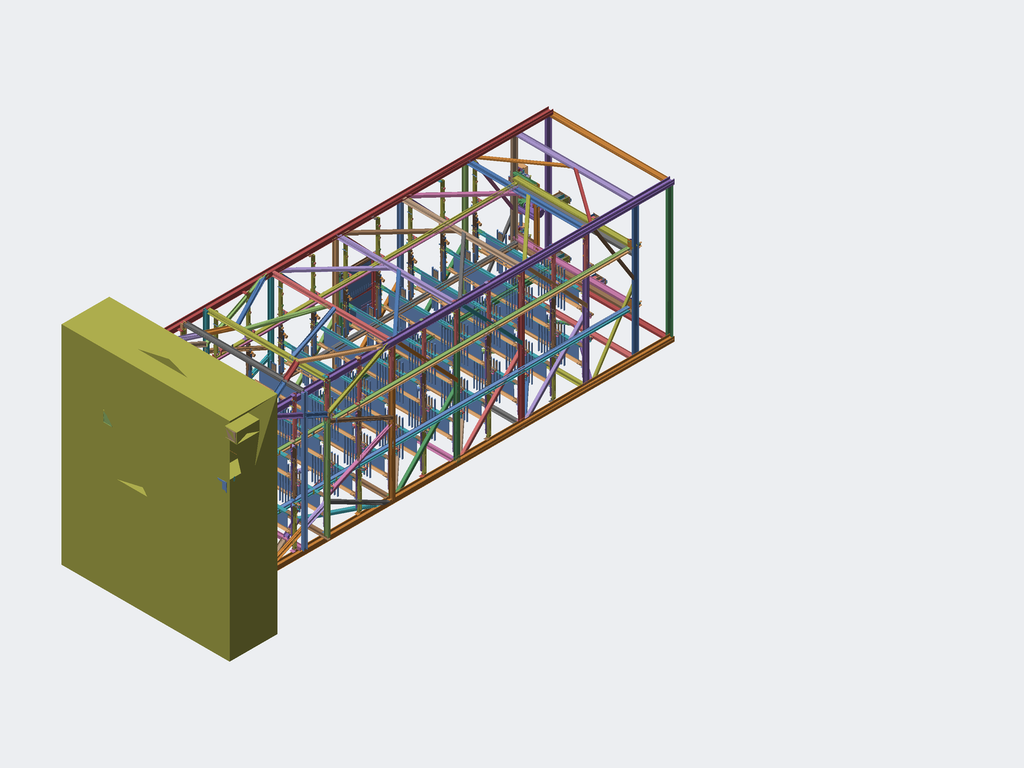Assembly | STEP file | 288 different items | 17335 placed
Parts list (item | name | quantity | parent item | size | volume):
1 | 01-Cross beam H150X150_default<machining> | x1 | in Main drive platform | 3170 x 150 x 150 mm | 12529220 mm3
2 | 01-Cross beam H150X150_default<machining> | x1 | in Main drive platform | 3170 x 150 x 150 mm | 12568854 mm3
3 | 02-Longitudinal beam H150X150_default<machining> | x1 | in Main drive platform | 1243 x 150 x 150 mm | 4402012 mm3
4 | 02-Longitudinal beam H150X150_default<machining> | x1 | in Main drive platform | 1243 x 150 x 150 mm | 4402012 mm3
5 | 02-Longitudinal beam H150X150_default<machining> | x1 | in Main drive platform | 1243 x 150 x 150 mm | 4482817 mm3
6 | 02-Longitudinal beam H150X150_default<machining> | x1 | in Main drive platform | 1243 x 150 x 150 mm | 4398211 mm3
7 | 02-Longitudinal beam H150X150_default<machining> | x1 | in Main drive platform | 1243 x 150 x 150 mm | 4398211 mm3
8 | Motor fixing plate | x1 | in Main drive platform | 370 x 435 x 20 mm | 3150576 mm3
9 | Bearing seat fixing plate | x2 | in Main drive platform | 470 x 360 x 20 mm | 3025589 mm3
10 | Counterweight hanging seat | x2 | in Main drive platform | 250 x 120 x 120 mm | 1060691 mm3
11 | 05 Rib plate | x4 | in Main drive platform | 176 x 140 x 10 mm | 160140 mm3
12 | 07 Rib plate | x2 | in Main drive platform | 156 x 140 x 10 mm | 146140 mm3
13 | 08 Rib plate | x2 | in Main drive platform | 166 x 140 x 10 mm | 153140 mm3
14 | 06 Rib plate | x4 | in Main drive platform | 71 x 128 x 10 mm | 86880 mm3
15 | 05-Base plate | x2 | in Sprocket seat | 360 x 470 x 16 mm | 2420472 mm3
16 | 04-Vertical plate | x4 | in Sprocket seat | 460 x 159 x 10 mm | 651900 mm3
17 | 03-Rib plate | x8 | in Sprocket seat | 152 x 159 x 10 mm | 208755 mm3
18 | 02-Top plate | x2 | in Sprocket seat | 460 x 550 x 16 mm | 3248676 mm3
19 | 01-Pad plate | x2 | in Sprocket seat | 148 x 110 x 6 mm | 92855 mm3
20 | 01-Pad plate | x2 | in Sprocket seat | 148 x 110 x 6 mm | 92855 mm3
21 | 01-Pad plate | x2 | in Sprocket seat | 148 x 110 x 6 mm | 92855 mm3
22 | 01-Pad plate | x2 | in Sprocket seat | 148 x 110 x 6 mm | 92855 mm3
23 | 06-Base plate | x8 | in Sprocket seat | 130 x 70 x 16 mm | 143137 mm3
24 | GB/T7810-1995 pillow block bearing UCP318 | x4 | in Drive mechanism assembly | 430 x 242.58 x 111.692 mm | 3436348 mm3
25 | 01-Main drive shaft | x2 | in Drive mechanism assembly | 1190 x 100 x 100 mm | 8433276 mm3
26 | Internal ring gear m=4  Z=56 | x2 | in CL7 Assembly | 180.99 x 350 x 350 mm | 2653491 mm3
27 | Internal ring gear A m=4  Z=56 | x2 | in CL7 Assembly | 177 x 350 x 350 mm | 2601765 mm3
28 | External ring gear m=4  Z=56 | x4 | in CL7 Assembly | 160.5 x 231.789 x 231.789 mm | 3084589 mm3
29 | Retaining ring | x4 | in CL7 Assembly | 19 x 240 x 240 mm | 192307 mm3
30 | Seal ring | x4 | in CL7 Assembly | 15.499 x 219.997 x 219.997 mm | 158146 mm3
31 | - | x4 | in CL7 Assembly | 3 x 239 x 239 mm | 65691 mm3
32 | Expansion ring | x4 | in CL7 Assembly | 245.982 x 245.031 x 3.5 mm | 25663 mm3
33 | Bolt M20x85 | x20 | in CL7 Assembly | 96 x 31.2 x 27.02 mm | 34962 mm3
34 | Grease fitting_M10X1_45 | x2 | in CL7 Assembly | 12 x 16.561 x 25.211 mm | 1753 mm3
35 | 03-Main drive sprocket | x2 | in Drive mechanism assembly | 232.271 x 231.883 x 162 mm | 2819895 mm3
36 | 02-Spacer | x4 | in Drive mechanism assembly | 100 x 100 x 22 mm | 32545 mm3
37 | Anti-jump chain bracket | x2 | in Drive mechanism assembly | 448 x 66 x 174 mm | 570819 mm3
38 | Chain press plate | x8 | in Drive mechanism assembly | 174 x 174 x 20 mm | 359243 mm3
39 | Anti-jump chain fixing seat | x1 | in Drive mechanism assembly | 550 x 308 x 360 mm | 1812248 mm3
40 | - | x2 | in Drive mechanism assembly | 70 x 27.713 x 24 mm | 16944 mm3
41 | - | x2 | in Drive mechanism assembly | 26.17 x 22.664 x 15.9 mm | 3864 mm3
42 | 01-Base plate | x2 | in Driven sprocket seat 1 | 420 x 16 x 435 mm | 2578914 mm3
43 | 03-Vertical plate | x2 | in Driven sprocket seat 1 | 420 x 204 x 16 mm | 1184293 mm3
44 | 03-Vertical plate | x2 | in Driven sprocket seat 1 | 420 x 204 x 16 mm | 1184293 mm3
45 | 02-Rib plate | x8 | in Driven sprocket seat 1 | 89 x 204 x 8 mm | 93564 mm3
46 | 04-Rib plate | x2 | in Driven sprocket seat 1 | 80 x 225 x 8 mm | 142200 mm3
47 | 04-Driven shaft 1 | x2 | in Driven sprocket assembly 1 | 305 x 60 x 60 mm | 857375 mm3
48 | PCSL50T-5300-03-Driven sprocket 1 | x2 | in Driven sprocket assembly 1 | 232.271 x 231.883 x 165 mm | 2210784 mm3
49 | GB/T276-94 deep groove ball bearing 6212-2Z | x8 | in Driven sprocket assembly 1, Driven sprocket assembly 2 | 22 x 110 x 110 mm | 94070 mm3
50 | GB893.1-86 hole elastic retaining ring type A 110 | x8 | in Driven sprocket assembly 1, Driven sprocket assembly 2 | 117 x 115.007 x 3 mm | 6744 mm3
51 | 05-Spacer 1 | x4 | in Driven sprocket assembly 1 | 70 x 70 x 39 mm | 39820 mm3
52 | Driven chain press plate 1 | x4 | in Driven sprocket assembly 1 | 130 x 170 x 20 mm | 254830 mm3
53 | Driven chain anti-jump bracket 1 | x2 | in Driven sprocket assembly 1 | 225 x 66 x 220 mm | 431717 mm3
54 | JBZQ4348-1997 shaft end baffle 60 | x8 | in Driven sprocket assembly 1, Driven sprocket assembly 2 | 130 x 40 x 8 mm | 37528 mm3
55 | Anti-jump chain fixing seat 1 | x1 | in Drive mechanism assembly | 550 x 308 x 360 mm | 1812248 mm3
56 | Counterweight connecting plate_default<machining> | x2 | in Drive mechanism assembly | 196 x 135 x 65 mm | 585213 mm3
57 | Chain joint | x8 | in Drive mechanism assembly | 40 x 65 x 25 mm | 47239 mm3
58 | - | x1 | in 209 | 694 x 505 x 541 mm | 76306472 mm3
59 | - | x1 | in 209 | 470 x 454.844 x 781 mm | 76496491 mm3
60 | 01-Top plate | x4 | - | 600 x 300 x 8 mm | 1430751 mm3
61 | 02-Base plate | x4 | - | 600 x 300 x 8 mm | 1412228 mm3
62 | 06-Middle plate | x2 | - | 600 x 442 x 8 mm | 2060678 mm3
63 | 03-Rib plate 1 | x4 | - | 146 x 419 x 6 mm | 366444 mm3
64 | 04-Rib plate 2 | x4 | - | 146 x 429 x 6 mm | 375204 mm3
65 | 05-Rib plate 3 | x4 | - | 146 x 439 x 6 mm | 383964 mm3
66 | 01-Gland cover 1 | x8 | - | 200 x 68 x 200 mm | 362165 mm3
67 | 02-Support strip | x32 | - | 200 x 22 x 12 mm | 50989 mm3
68 | 04-Middle plate | x2 | - | 600 x 348 x 8 mm | 1609674 mm3
69 | 01-Rib plate 1 | x4 | - | 146 x 325 x 6 mm | 284100 mm3
70 | 02-Rib plate 2 | x4 | - | 146 x 335 x 6 mm | 292860 mm3
71 | 03-Rib plate 3 | x4 | - | 146 x 345 x 6 mm | 301620 mm3
72 | 01-Base plate 1 | x2 | in Driven sprocket seat 2 | 420 x 16 x 435 mm | 2714914 mm3
73 | 03-Vertical plate 1 | x2 | in Driven sprocket seat 2 | 420 x 224 x 16 mm | 1446053 mm3
74 | 03-Vertical plate 1 | x2 | in Driven sprocket seat 2 | 420 x 224 x 16 mm | 1446053 mm3
75 | 02-Rib plate 1 | x8 | in Driven sprocket seat 2 | 112 x 224 x 8 mm | 124732 mm3
76 | 04-Rib plate 1 | x2 | in Driven sprocket seat 2 | 120 x 178 x 8 mm | 169080 mm3
77 | 04-Driven shaft 2 | x2 | in Driven sprocket assembly 2 | 258 x 60 x 60 mm | 726613 mm3
78 | 03-Driven sprocket 2 | x2 | in Driven sprocket assembly 2 | 232.271 x 231.883 x 81 mm | 1194859 mm3
79 | 05-Spacer 2 | x4 | in Driven sprocket assembly 2 | 70 x 70 x 57.5 mm | 58709 mm3
80 | 01-Driven chain press plate 2 | x4 | in Driven sprocket assembly 2 | 164 x 204 x 20 mm | 376718 mm3
81 | 02-Driven chain anti-jump bracket 2 | x2 | in Driven sprocket assembly 2 | 178 x 66 x 254 mm | 427046 mm3
82 | chain_16a inner link | x12120 | in Chain 2, Chain 1, Assembly 3 | 49.4 x 24 x 22.25 mm | 10373 mm3
83 | 01-Column (flat tube 200x100x8)_default<machining> | x6 | in Fixed base frame | 1300 x 100 x 200 mm | 5692942 mm3
84 | 02-Cross beam (flat tube 200x100x8)_default<machining> | x2 | in Fixed base frame | 6536 x 100 x 200 mm | 28622358 mm3
85 | 03-Longitudinal beam (flat tube 200x100x8)_default<machining> | x8 | in Fixed base frame | 670 x 100 x 200 mm | 2934054 mm3
86 | 04-Steel plate | x2 | in Fixed base frame | 1888 x 300 x 12 mm | 6796800 mm3
87 | 05-Longitudinal beam (flat tube 200x100x8)_default<machining> | x4 | in Fixed base frame | 509 x 100 x 200 mm | 2229006 mm3
88 | 06-Channel 100x48_default<machining> | x2 | in Fixed base frame | 670 x 48 x 100 mm | 842936 mm3
89 | 07-Channel 100x48_default<machining> | x4 | in Fixed base frame | 509 x 65 x 160 mm | 1267662 mm3
90 | 08-Channel 100x48_default<machining> | x2 | in Fixed base frame | 2320 x 65 x 160 mm | 5777947 mm3
91 | 09-Bent plate | x4 | in Fixed base frame | 65 x 65 x 86.5 mm | 83900 mm3
92 | 12-(flat tube 200x100x8)_default<machining> | x4 | in Fixed base frame | 150 x 100 x 200 mm | 656878 mm3
93 | 14-Pad plate | x4 | in Fixed base frame | 100 x 150 x 20 mm | 300000 mm3
94 | 13-Positioning switch bracket | x4 | in Fixed base frame | 38 x 103 x 80 mm | 41502 mm3
95 | 01-Positioning block seat | x2 | in Positioning stopper | 40 x 67 x 85 mm | 64658 mm3
96 | 02-Rubber pad | x2 | in Positioning stopper | 40 x 85 x 15 mm | 48295 mm3
97 | 11-Bent plate | x4 | in Fixed base frame | 65 x 65 x 491 mm | 493529 mm3
98 | 11-Bent plate (symmetric) | x4 | in Fixed base frame | 65 x 65 x 491 mm | 493529 mm3
99 | 10-Bent plate | x4 | in Fixed base frame | 65 x 65 x 172 mm | 170584 mm3
100 | 15-Steel plate | x1 | in Fixed base frame | 400 x 300 x 16 mm | 1845004 mm3
101 | 01-Channel 160x65(symmetric)_default<machining> | x1 | in First-level parking platform | 4896 x 65 x 160 mm | 11823421 mm3
102 | 01-Channel 160x65(symmetric)_default<machining> | x1 | in First-level parking platform | 4896 x 65 x 160 mm | 11823421 mm3
103 | 02-Channel 100x48_default<machining> | x8 | in First-level parking platform | 505 x 48 x 100 mm | 635347 mm3
104 | 03-Side middle pedal | x2 | in First-level parking platform | 104 x 510 x 600 mm | 1457819 mm3
105 | 05-Channel 160x65_default<machining> | x1 | in First-level parking platform | 853 x 65 x 160 mm | 1957806 mm3
106 | 05-Channel 160x65_default<machining> | x1 | in First-level parking platform | 853 x 65 x 160 mm | 1957807 mm3
107 | 04-Base plate | x1 | in First-level parking platform | 400 x 300 x 16 mm | 1829151 mm3
108 | - | x20 | in First-level parking platform | 1888 x 30 x 60 mm | 1160736 mm3
109 | 07-Rib plate | x2 | in First-level parking platform | 1440 x 60 x 4 mm | 345600 mm3
110 | 08-Middle cover plate | x2 | in First-level parking platform | 1252 x 870 x 4 mm | 4356960 mm3
111 | 09-End cover plate | x2 | in First-level parking platform | 714.448 x 870 x 4 mm | 2441819 mm3
112 | 10-Side end pedal | x2 | in First-level parking platform | 521.6 x 509 x 4 mm | 931106 mm3
113 | 10-Side end pedal (symmetric) | x2 | in First-level parking platform | 521.6 x 509 x 4 mm | 931106 mm3
114 | 11-Channel 100x48_default<machining> | x4 | in First-level parking platform | 355 x 48 x 100 mm | 375001 mm3
115 | 12-Channel 100x48_default<machining> | x4 | in First-level parking platform | 544 x 48 x 100 mm | 666800 mm3
116 | 13-Steel plate | x4 | in First-level parking platform | 349 x 220 x 10 mm | 697400 mm3
117 | 16-Steel plate | x2 | in First-level parking platform | 350 x 740 x 10 mm | 2590000 mm3
118 | 17-Reinforcing bent plate 1 | x40 | in First-level parking platform | 38 x 34 x 459 mm | 170472 mm3
119 | 18-Reinforcing bent plate 2 | x3 | in First-level parking platform | 38 x 34 x 50 mm | 17215 mm3
120 | 19B-Reinforcing bent plate 2 | x6 | in First-level parking platform | 38 x 34 x 50 mm | 17215 mm3
121 | 19B-Reinforcing bent plate 21 | x3 | in First-level parking platform | 38 x 34 x 50 mm | 17215 mm3
122 | 19-Side baffle 1 | x1 | in First-level parking platform | 190.691 x 1891 x 160 mm | 983357 mm3
123 | 24B-Side baffle 2 | x1 | in First-level parking platform | 190.691 x 1891 x 160 mm | 813219 mm3
124 | 20-Positioning block | x2 | in First-level parking platform | 25 x 30 x 20 mm | 15000 mm3
125 | 21-Guide positioning block | x4 | in First-level parking platform | 76.059 x 76.059 x 27.6 mm | 24483 mm3
126 | Photoelectric bracket 2 | x4 | in First-level parking platform | 22 x 62 x 58 mm | 7067 mm3
127 | Through-beam photoelectric sensor | x4 | in First-level parking platform | 52.612 x 52.612 x 18 mm | 43705 mm3
128 | 05-Switch striker | x2 | in First-level parking platform | 31 x 230 x 40 mm | 29136 mm3
129 | 05-Channel 160x65_default<machining> | x2 | in First-level parking platform | 853 x 65 x 160 mm | 1958415 mm3
130 | - | x4 | in First-level parking platform | 10.89 x 9.431 x 6.4 mm | 311.158 mm3
131 | GB/T7810-1995 square flange bearing UCFU216 | x1 | in First-level parking platform assembly | 213 x 213 x 84.7 mm | 1127031 mm3
132 | 01 End cover plate | x2 | in First-level parking platform assembly | 300 x 866 x 4 mm | 1037390 mm3
133 | 02 Middle cover plate | x1 | in First-level parking platform assembly | 480 x 866 x 4 mm | 1660910 mm3
134 | Cover plate | x1 | in First-level parking platform assembly | 6576 x 4 x 3300 mm | 20991561 mm3
135 | 04-H125X125X6.5X9_default<machining> | x1 | in Counterweight frame | 2916 x 125 x 125 mm | 8741134 mm3
136 | 04-H125X125X6.5X9_default<machining> | x1 | in Counterweight frame | 2916 x 125 x 125 mm | 8749277 mm3
137 | 01-H125X125X6.5X9_default<machining> | x1 | in Counterweight frame | 125 x 125 x 1610 mm | 4827397 mm3
138 | 01-H125X125X6.5X9_default<machining> | x1 | in Counterweight frame | 125 x 125 x 1610 mm | 4827397 mm3
139 | 02-Steel plate | x5 | in Counterweight frame | 110 x 1860 x 10 mm | 2046000 mm3
140 | 03-Reinforcing rib plate | x4 | in Counterweight frame | 215 x 215 x 10 mm | 421750 mm3
141 | 05-Connecting plate | x2 | in Counterweight frame | 110 x 105 x 10 mm | 112421 mm3
142 | 06-Reinforcing rib plate | x4 | in Counterweight frame | 215 x 90 x 10 mm | 153000 mm3
143 | Hanging sprocket seat | x2 | in Counterweight frame | 150 x 176 x 220 mm | 1392367 mm3
144 | 08-Rib plate | x8 | in Counterweight frame | 59 x 105 x 8 mm | 48760 mm3
145 | 03-Counterweight block pressure iron 2_default<machining> | x2 | in Counterweight device | 90 x 100 x 63 mm | 80067 mm3
146 | Guide shoe upper bracket | x2 | in Counterweight device | 149 x 168 x 96 mm | 228852 mm3
147 | Guide shoe lower bracket | x2 | in Counterweight device | 120 x 101 x 136 mm | 190804 mm3
148 | Connecting plate | x1 | in Counterweight device | 110 x 1805 x 10 mm | 1957224 mm3
149 | 05-Sprocket shaft | x2 | in Counterweight device | 40 x 235 x 40 mm | 293750 mm3
150 | 07-Sprocket | x2 | in Counterweight device | 150.693 x 150.061 x 162 mm | 851897 mm3
151 | GB/T276-94 deep groove ball bearing 6208-2Z | x4 | in Counterweight device | 18 x 80 x 80 mm | 42698 mm3
152 | GB893.1-86 hole elastic retaining ring type A 80 | x4 | in Counterweight device | 85.5 x 83.408 x 2.5 mm | 3180 mm3
153 | 06-Spacer | x4 | in Counterweight device | 47 x 17 x 47 mm | 8131 mm3
154 | 08-Baffle | x2 | in Counterweight device | 80 x 40 x 6 mm | 17353 mm3
155 | 09-Protective cover | x2 | in Counterweight device | 210 x 81.361 x 90 mm | 57744 mm3
156 | 01 Counterweight block | x148 | in Counterweight device | 124 x 1345 x 20 mm | 3242800 mm3
157 | TK5 guide rail single shoe head | x4 | in Counterweight device | 110 x 85 x 51.5 mm | 179270 mm3
158 | - | x1 | - | 5334 x 100 x 200 mm | 23358303 mm3
159 | 01-Connecting plate 1 | x2 | - | 180 x 230 x 25 mm | 971744 mm3
160 | 03-High-level comb rack 1 | x8 | - | 90 x 507 x 36 mm | 1352906 mm3
161 | 06-Steel plate 680x180x8 | x1 | - | 680 x 180 x 8 mm | 916480 mm3
162 | 08-Steel plate 130x50x8 | x1 | - | 130 x 50 x 8 mm | 52000 mm3
163 | 09-Steel plate 25x65x6 | x1 | - | 25 x 65 x 6 mm | 9750 mm3
164 | 10-Part 25x100x6 | x1 | - | 25 x 100 x 6 mm | 15000 mm3
165 | 07-High-level comb rack 3 | x1 | - | 90 x 507 x 36 mm | 1363460 mm3
166 | 04-Steel plate 680x180x8 | x1 | - | 680 x 180 x 8 mm | 979200 mm3
167 | 05-Steel plate 825x180x8 | x1 | - | 825 x 180 x 8 mm | 1188000 mm3
168 | 01-Bent plate 11 | x11 | in Comb rack II | 505.277 x 100 x 20 mm | 220935 mm3
169 | 02-Bent plate 2 | x11 | in Comb rack II | 505.277 x 100 x 20 mm | 220935 mm3
170 | 03-Sealing plate | x11 | in Comb rack II | 34 x 57 x 2 mm | 3876 mm3
171 | 01B-Bent plate 11 | x11 | in 00-Comb rack II, 00-Comb rack II-1, 00-Comb rack II-2, 00-Comb rack II-3, 00-Comb rack II-4, 00-Comb rack II-5 | 505.277 x 100 x 20 mm | 220935 mm3
172 | 02B-Bent plate 2 | x11 | in 00-Comb rack II, 00-Comb rack II-1, 00-Comb rack II-2, 00-Comb rack II-3, 00-Comb rack II-4, 00-Comb rack II-5 | 505.277 x 100 x 20 mm | 220935 mm3
173 | 03B-Sealing plate | x11 | in 00-Comb rack II, 00-Comb rack II-1, 00-Comb rack II-2, 00-Comb rack II-3, 00-Comb rack II-4, 00-Comb rack II-5 | 34 x 57 x 2 mm | 3876 mm3
174 | 03-High-level comb rack 11 | x8 | in Main beam I (symmetric) | 90 x 507 x 36 mm | 1352907 mm3
175 | 06B-Part 6 | x1 | in Main beam I (symmetric) | 825 x 180 x 8 mm | 1188000 mm3
176 | 02B-Square tube 200x100x8_default<machining> | x1 | in Main beam I (symmetric) | 5334 x 100 x 200 mm | 23358303 mm3
177 | 01-Connecting plate 11 | x2 | in Main beam I (symmetric) | 180 x 230 x 25 mm | 971744 mm3
178 | - | x1 | in Main beam I (symmetric) | 680 x 180 x 8 mm | 916480 mm3
179 | - | x1 | in Main beam I (symmetric) | 130 x 50 x 8 mm | 52000 mm3
180 | 10B-Part 10 | x1 | in Main beam I (symmetric) | 25 x 65 x 6 mm | 9750 mm3
181 | 11B-Part 11 | x1 | in Main beam I (symmetric) | 25 x 100 x 6 mm | 15000 mm3
182 | 08-High-level comb rack 3 | x1 | in Main beam I (symmetric) | 90 x 507 x 36 mm | 1363460 mm3
183 | - | x1 | in Main beam I (symmetric) | 680 x 180 x 8 mm | 979200 mm3
184 | 05-Vertical plate 1 | x2 | in Fork arm 2 | 16 x 158 x 703 mm | 1685184 mm3
185 | 05-Vertical plate 1 | x2 | in Fork arm 2 | 16 x 158 x 703 mm | 1685184 mm3
186 | 04-Square plate | x8 | in Fork arm 2, Fork arm 2 (symmetric) | 47.5 x 158 x 16 mm | 120080 mm3
187 | 03-Plate 1 | x2 | in Fork arm 2 | 158 x 475 x 25 mm | 1521139 mm3
188 | 01-Top plate 1 | x4 | in Fork arm 2, Fork arm 2 (symmetric) | 120 x 158 x 20 mm | 360030 mm3
189 | 02-Reinforcing rib 13 | x16 | in Fork arm 2, Fork arm 2 (symmetric) | 47.5 x 83 x 10 mm | 28013 mm3
190 | 07-Square plate | x4 | in Fork arm 2, Fork arm 2 (symmetric) | 158 x 120 x 16 mm | 303360 mm3
191 | 08-Plate 2 | x2 | in Fork arm 2 | 128 x 172.5 x 25 mm | 507364 mm3
192 | 06-Square plate | x8 | in Fork arm 2, Fork arm 2 (symmetric) | 703 x 78 x 10 mm | 548340 mm3
193 | - | x2 | in Fork arm 2 | 352 x 230 x 382 mm | 4009392 mm3
194 | 04-Spacer 1 | x8 | in Guide column II, Guide column II (symmetric) | 48 x 48 x 19.5 mm | 8270 mm3
195 | 02-Guide roller 2 | x16 | in Guide column II, Guide column II (symmetric) | 40 x 175 x 175 mm | 657116 mm3
196 | GB/T276-94 deep groove ball bearing 6308-2Z | x16 | in Guide column II, Guide column II (symmetric) | 23 x 90 x 90 mm | 71674 mm3
197 | GB893.1-86 hole elastic retaining ring type A 90 | x12 | in Guide column II, Guide column II (symmetric) | 95.5 x 93.873 x 2.5 mm | 3834 mm3
198 | GB894.2-86 shaft elastic retaining ring type B 40 | x16 | in Guide column II, Guide column II (symmetric) | 44 x 48.437 x 1.5 mm | 802.829 mm3
199 | 03-Pin shaft 1 | x8 | in Guide column II, Guide column II (symmetric) | 49 x 121.4 x 49 mm | 170065 mm3
200 | 05-Vertical plate 1 | x2 | in Fork arm 2 (symmetric) | 16 x 158 x 703 mm | 1685184 mm3
201 | 05-Vertical plate 1 | x2 | in Fork arm 2 (symmetric) | 16 x 158 x 703 mm | 1685184 mm3
202 | 03-Plate 1 | x2 | in Fork arm 2 (symmetric) | 158 x 475 x 25 mm | 1521139 mm3
203 | 08-Plate 2 | x2 | in Fork arm 2 (symmetric) | 128 x 172.5 x 25 mm | 507364 mm3
204 | - | x2 | in Fork arm 2 (symmetric) | 352 x 230 x 382 mm | 4009542 mm3
205 | Lifting fork tie rod | x4 | in Lifting fork assembly | 60 x 213 x 24 mm | 148905 mm3
206 | Lifting fork connecting plate 2_default<machining> | x4 | in Lifting fork assembly | 160 x 110 x 65 mm | 490207 mm3
207 | 14-Chain joint | x8 | in Lifting fork assembly | 40 x 65 x 25 mm | 47239 mm3
208 | 02 Bent plate | x4 | in Lifting fork assembly | 30 x 120 x 120 mm | 44037 mm3
209 | - | x1 | in Lifting fork assembly | 68 x 16 x 16 mm | 7681 mm3
210 | Adjusting shim 1 | x1 | in Lifting fork assembly | 87 x 230 x 1 mm | 16008 mm3
211 | Concrete | x1 | - | 11000 x 2521 x 8890 mm | 220029236509 mm3
212 | Steel structure_default<machining> | x1 | - | - | 3257360996 mm3
213 | 012-Rectangular tube 150x100x8_default<machining> | x20 | - | 2470 x 100 x 150 mm | 8324006 mm3
214 | - | x20 | - | 210 x 71 x 192 mm | 470787 mm3
215 | 02-Square plate 1 | x60 | - | 220 x 40 x 12 mm | 91800 mm3
216 | 02-Support shaft 1 | x80 | - | 173.5 x 35 x 35 mm | 161107 mm3
217 | 01-Support roller | x80 | - | 30 x 100 x 100 mm | 201135 mm3
218 | GB/T276-94 deep groove ball bearing 6207-N | x360 | in Roller support II, Roller support VII | 17 x 72 x 72 mm | 35893 mm3
219 | 01-Spacer 1 | x180 | in Roller support II, Roller support VII | 42 x 27 x 42 mm | 11430 mm3
220 | GB894.2-86 shaft elastic retaining ring type B 35 | x180 | in Roller support II, Roller support VII | 39 x 42.531 x 1.5 mm | 639.019 mm3
221 | 02-Support shaft 5 | x40 | - | 226.5 x 35 x 35 mm | 210864 mm3
222 | 01-Support roller 5 | x40 | - | 30 x 100 x 100 mm | 201135 mm3
223 | 02-Support shaft 3 | x40 | - | 286.5 x 35 x 35 mm | 267927 mm3
224 | 01-Support roller 2 | x40 | - | 30 x 100 x 100 mm | 201135 mm3
225 | 03-Small sprocket 1 | x100 | in Roller support II, Roller support VII | 83.551 x 83.273 x 25 mm | 37685 mm3
226 | 02-Spacer 2 | x60 | in Roller support II, Roller support VII | 42 x 42 x 3 mm | 1270 mm3
227 | 05-Spacer 3 | x40 | in Roller support II, Roller support VII | 42 x 42 x 60 mm | 25400 mm3
228 | 01-Seat plate 1 | x40 | in Roller seat I | 130 x 150 x 6 mm | 108788 mm3
229 | 02-Support shaft 4 | x40 | in Roller seat I | 22 x 35 x 22 mm | 9653 mm3
230 | 04-Small sprocket 2 | x60 | in Roller support II, Roller seat II, Roller support VII | 50.563 x 50.061 x 15 mm | 10157 mm3
231 | SF-1 oil-free bearing 1615 | x60 | in Roller support II, Roller seat II, Roller support VII | 18 x 18 x 15 mm | 789.176 mm3
232 | GB894.1-86 shaft elastic retaining ring type A 16 | x40 | in Roller support II, Roller support VII | 18.2 x 20.685 x 1 mm | 106.213 mm3
233 | Motor IPL22-200-30 | x40 | in Roller support II, Roller support VII | 157.5 x 145 x 294.5 mm | 3005281 mm3
234 | 06-Small sprocket 4 | x40 | in Roller support II, Roller support VII | 91.703 x 91.451 x 30 mm | 58578 mm3
235 | Motor chain 1 | x40 | in Roller support II, Roller support VII | 321.643 x 97.927 x 16.175 mm | 70929 mm3
236 | 01-Seat plate 2 | x20 | in Roller seat II | 130 x 150 x 6 mm | 108788 mm3
237 | 02-Support shaft 21 | x20 | in Roller seat II | 22 x 60 x 22 mm | 19156 mm3
238 | 02-Small sprocket 3 | x40 | in Roller support II | 83.535 x 83.254 x 31.985 mm | 63279 mm3
239 | 01-Spacer 51 | x40 | in Roller support II | 42 x 42 x 20.6 mm | 8721 mm3
240 | Middle chain 2 | x40 | in Roller support II | - | 129311 mm3
241 | 011-Rectangular tube 150x100x8_default<machining> | x20 | - | 2098 x 100 x 150 mm | 7060017 mm3
242 | - | x20 | - | 210 x 71 x 192 mm | 470787 mm3
243 | 02-Support shaft 2 | x20 | - | 201.5 x 35 x 35 mm | 187096 mm3
244 | 01-Support roller 1 | x20 | - | 30 x 100 x 100 mm | 201135 mm3
245 | Middle chain | x20 | in Roller support VII | 605.495 x 93.494 x 16.175 mm | 126775 mm3
246 | Mirror 011-rectangular tube 150x100x8_default<machining> | x20 | - | 2098 x 100 x 150 mm | 7060017 mm3
247 | - | x20 | - | 210 x 71 x 192 mm | 470787 mm3
248 | Mirror 02-Square plate 1 | x20 | - | 220 x 40 x 12 mm | 91800 mm3
249 | Mirror 02-Support shaft 1 | x40 | - | 173.5 x 35 x 35 mm | 161107 mm3
250 | Mirror 01-Support roller | x40 | - | 30 x 100 x 100 mm | 201135 mm3
251 | Mirror GB/T276-94 deep groove ball bearing 6207-N | x160 | in Mirror roller support VII | 17 x 72 x 72 mm | 35895 mm3
252 | Mirror 01-Spacer 1 | x80 | in Mirror roller support VII | 42 x 27 x 42 mm | 11430 mm3
253 | Mirror GB894.2-86 shaft elastic retaining ring type B 35 | x80 | in Mirror roller support VII | 39 x 42.531 x 1.5 mm | 639.019 mm3
254 | Mirror 02-Support shaft 2 | x20 | - | 201.5 x 35 x 35 mm | 187096 mm3
255 | Mirror 01-Support roller 1 | x20 | - | 30 x 100 x 100 mm | 201135 mm3
256 | Mirror 02-Spacer 2 | x40 | in Mirror roller support VII | 42 x 42 x 3 mm | 1270 mm3
257 | Mirror 03-Small sprocket 1 | x60 | in Mirror roller support VII | 83.551 x 83.273 x 25 mm | 37685 mm3
258 | Mirror 02-Support shaft 3 | x20 | - | 286.5 x 35 x 35 mm | 267926 mm3
259 | Mirror 01-Support roller 2 | x20 | - | 30 x 100 x 100 mm | 201135 mm3
260 | Mirror 05-Spacer 3 | x20 | in Mirror roller support VII | 42 x 42 x 60 mm | 25400 mm3
261 | Mirror 01-Seat plate 1 | x20 | - | 130 x 150 x 6 mm | 108788 mm3
262 | Mirror 02-Support shaft 4 | x20 | - | 22 x 35 x 22 mm | 9653 mm3
263 | Mirror 04-Small sprocket 2 | x20 | in Mirror roller support VII | 50.563 x 50.061 x 15 mm | 10157 mm3
264 | Mirror SF-1 oil-free bearing 1615 | x20 | in Mirror roller support VII | 18 x 18 x 15 mm | 789.176 mm3
265 | Mirror GB894.1-86 shaft elastic retaining ring type A 16 | x20 | in Mirror roller support VII | 18.2 x 20.685 x 1 mm | 106.213 mm3
266 | Mirror motor IPL22-200-30 | x20 | in Mirror roller support VII | 157.5 x 145 x 294.5 mm | 3005281 mm3
267 | Mirror 06-Small sprocket 4 | x20 | in Mirror roller support VII | 91.703 x 91.451 x 30 mm | 58578 mm3
268 | Mirror motor chain 1 | x20 | in Mirror roller support VII | 321.643 x 97.927 x 16.175 mm | 70929 mm3
269 | Mirror middle chain | x20 | in Mirror roller support VII | 605.495 x 93.494 x 16.175 mm | 126775 mm3
270 | 05-Left main beam 1_default<machining> | x20 | - | 5344 x 65 x 160 mm | 13076241 mm3
271 | 01-Right main beam 1_default<machining> | x20 | - | 5344 x 65 x 160 mm | 13076241 mm3
272 | 02-Rectangular tube 60x30x4_default<machining> | x300 | - | 1880 x 30 x 60 mm | 1155817 mm3
273 | 03-Support plate | x40 | - | 420 x 65 x 6 mm | 163800 mm3
274 | 04-Support plate | x40 | - | 1020 x 65 x 6 mm | 397800 mm3
275 | 06-Reinforcing bent plate 1 | x280 | - | 38 x 34 x 50 mm | 17557 mm3
276 | 07-Reinforcing bent plate 2 | x280 | - | 38 x 34 x 459 mm | 161170 mm3
277 | - | x20 | - | 78.969 x 125 x 1880 mm | 3813981 mm3
278 | 02-Reinforcing rib 1 | x80 | - | 100 x 140 x 6 mm | 48661 mm3
279 | 03-Connecting plate 1 | x40 | - | 350 x 160 x 16 mm | 757922 mm3
280 | 04-Travel stopper | x20 | - | 100 x 30 x 10 mm | 30000 mm3
281 | - | x20 | - | 78.969 x 125 x 1880 mm | 3813981 mm3
282 | 03-Connecting plate 11 | x40 | - | 350 x 160 x 16 mm | 757922 mm3
283 | 02-Reinforcing rib 11 | x80 | - | 100 x 140 x 6 mm | 48661 mm3
284 | 00B-Travel stopper | x20 | - | 100 x 30 x 10 mm | 30000 mm3
285 | 01-Bent plate 1 | x40 | - | 18.464 x 131.962 x 40 mm | 22033 mm3
286 | 02-Angle steel 30x30x3_default<machining> | x40 | - | 67 x 30 x 30 mm | 11719 mm3
287 | 03-Stick plate 1 | x40 | - | 63.208 x 109.115 x 80 mm | 34953 mm3
288 | 01-Cover plate | x20 | in 193 | 4900 x 0.6 x 870 mm | 2557612 mm3
Placements (level | parent | child | x y z in mm | rotation matrix by rows), first 242 of 17995 lines:
1 | subassembly 2 | Lifting drive and platform | -1237.622 -17108.525 26506.0 | 1 0 0 0 1 0 0 0 1
2 | Lifting drive and platform | Drive mechanism assembly | -2872.5 23245.273 -39.393 | 0 0 1 0 1 0 -1 0 0
3 | Drive mechanism assembly | Main drive platform | -66.906 28.577 -572.5 | 1 0 0 0 1 0 0 0 1
4 | Main drive platform | 01-Cross beam H150X150_default<machining> | -1557.487 16.15 -0.0 | 1 0 0 0 1 0 0 0 1
4 | Main drive platform | 01-Cross beam H150X150_default<machining> | -1557.487 16.15 1250.0 | 1 0 0 0 1 0 0 0 1
4 | Main drive platform | 02-Longitudinal beam H150X150_default<machining> | -1482.487 16.15 1246.5 | 0 -1 0 0 0 1 -1 0 0
4 | Main drive platform | 02-Longitudinal beam H150X150_default<machining> | -1162.487 16.15 1246.5 | 0 -1 0 0 0 1 -1 0 0
4 | Main drive platform | 02-Longitudinal beam H150X150_default<machining> | 27.513 16.15 1246.5 | 0 -1 0 0 0 1 -1 0 0
4 | Main drive platform | 02-Longitudinal beam H150X150_default<machining> | 1217.513 16.15 1246.5 | 0 -1 0 0 0 1 -1 0 0
4 | Main drive platform | 02-Longitudinal beam H150X150_default<machining> | 1537.513 16.15 1246.5 | 0 -1 0 0 0 1 -1 0 0
4 | Main drive platform | Motor fixing plate | -157.487 91.15 -160.0 | 1 0 0 0 0 1 0 -1 0
4 | Main drive platform | Bearing seat fixing plate | -1557.487 91.15 -180.0 | 1 0 0 0 0 1 0 -1 -0
4 | Main drive platform | Bearing seat fixing plate | 1142.513 91.15 -180.0 | 1 0 0 0 0 1 0 -1 -0
4 | Main drive platform | Counterweight hanging seat | 1262.513 -70.85 -55.0 | 1 0 0 0 1 0 0 0 1
4 | Main drive platform | Counterweight hanging seat | -1437.487 -70.85 -55.0 | 1 0 0 0 1 0 0 0 1
4 | Main drive platform | 05 Rib plate | -1477.487 91.15 -179.5 | 0 0 -1 0 1 0 1 0 0
4 | Main drive platform | 05 Rib plate | -1157.487 91.15 -179.5 | 0 0 -1 0 1 0 1 0 0
4 | Main drive platform | 07 Rib plate | 107.513 91.15 -159.5 | 0 0 -1 0 1 0 1 0 0
4 | Main drive platform | 07 Rib plate | -42.487 91.15 -159.5 | 0 0 -1 0 1 0 1 0 0
4 | Main drive platform | 05 Rib plate | 1542.513 91.15 -179.5 | 0 0 -1 0 1 0 1 0 0
4 | Main drive platform | 05 Rib plate | 1222.513 91.15 -179.5 | 0 0 -1 0 1 0 1 0 0
4 | Main drive platform | 08 Rib plate | -141.987 91.15 240.0 | 1 0 0 0 1 0 0 0 1
4 | Main drive platform | 08 Rib plate | 197.013 91.15 250.0 | -1 0 0 0 1 0 0 0 -1
4 | Main drive platform | 06 Rib plate | -572.487 80.15 1324.5 | 0 0 1 0 1 0 -1 0 -0
4 | Main drive platform | 06 Rib plate | 617.513 80.15 1324.5 | 0 0 1 0 1 0 -1 0 -0
4 | Main drive platform | 06 Rib plate | -562.487 80.15 -74.5 | 0 0 -1 0 1 0 1 0 0
4 | Main drive platform | 06 Rib plate | 627.513 80.15 -74.5 | 0 0 -1 0 1 0 1 0 0
3 | Drive mechanism assembly | Sprocket seat | -1632.393 155.727 -540.358 | 0 0 -1 0 1 0 1 0 -0
4 | Sprocket seat | 05-Base plate | -212.142 -0.0 -8.0 | 1 0 0 0 0 -1 0 1 0
4 | Sprocket seat | 04-Vertical plate | -262.142 159.0 -130.5 | 1 0 0 0 1 0 0 0 1
4 | Sprocket seat | 04-Vertical plate | -262.142 159.0 -365.5 | 1 0 0 0 1 0 0 0 1
4 | Sprocket seat | 03-Rib plate | 67.858 159.0 -120.5 | 0 0 -1 0 1 0 1 0 -0
4 | Sprocket seat | 03-Rib plate | -122.142 159.0 -120.5 | 0 0 -1 0 1 0 1 0 -0
4 | Sprocket seat | 03-Rib plate | 57.858 159.0 -365.5 | 0 0 1 0 1 0 -1 0 0
4 | Sprocket seat | 03-Rib plate | -132.142 159.0 -365.5 | 0 0 1 0 1 0 -1 0 0
4 | Sprocket seat | 02-Top plate | 197.858 159.0 32.0 | -1 0 0 0 0 1 0 1 -0
4 | Sprocket seat | 01-Pad plate | 49.858 181.0 -28.0 | 1 0 0 0 0 -1 0 1 -0
4 | Sprocket seat | 01-Pad plate | 49.858 181.0 -348.0 | 1 0 0 0 0 -1 0 1 -0
4 | Sprocket seat | 01-Pad plate | -262.142 181.0 -28.0 | 1 0 0 0 0 -1 0 1 -0
4 | Sprocket seat | 01-Pad plate | -262.142 181.0 -348.0 | 1 0 0 0 0 -1 0 1 -0
4 | Sprocket seat | 06-Base plate | 213.858 229.0 -148.0 | 0 0 -1 0 1 0 1 0 -0
4 | Sprocket seat | 06-Base plate | 213.858 229.0 -468.0 | 0 0 -1 0 1 0 1 0 -0
4 | Sprocket seat | 06-Base plate | -262.142 229.0 -148.0 | 0 0 -1 0 1 0 1 0 -0
4 | Sprocket seat | 06-Base plate | -262.142 229.0 -468.0 | 0 0 -1 0 1 0 1 0 -0
3 | Drive mechanism assembly | Sprocket seat | 1067.607 155.727 -540.358 | 0 0 -1 0 1 0 1 0 -0
4 | Sprocket seat | 05-Base plate | -212.142 -0.0 -8.0 | 1 0 0 0 0 -1 0 1 0
4 | Sprocket seat | 04-Vertical plate | -262.142 159.0 -130.5 | 1 0 0 0 1 0 0 0 1
4 | Sprocket seat | 04-Vertical plate | -262.142 159.0 -365.5 | 1 0 0 0 1 0 0 0 1
4 | Sprocket seat | 03-Rib plate | 67.858 159.0 -120.5 | 0 0 -1 0 1 0 1 0 -0
4 | Sprocket seat | 03-Rib plate | -122.142 159.0 -120.5 | 0 0 -1 0 1 0 1 0 -0
4 | Sprocket seat | 03-Rib plate | 57.858 159.0 -365.5 | 0 0 1 0 1 0 -1 0 0
4 | Sprocket seat | 03-Rib plate | -132.142 159.0 -365.5 | 0 0 1 0 1 0 -1 0 0
4 | Sprocket seat | 02-Top plate | 197.858 159.0 32.0 | -1 0 0 0 0 1 0 1 -0
4 | Sprocket seat | 01-Pad plate | 49.858 181.0 -28.0 | 1 0 0 0 0 -1 0 1 -0
4 | Sprocket seat | 01-Pad plate | 49.858 181.0 -348.0 | 1 0 0 0 0 -1 0 1 -0
4 | Sprocket seat | 01-Pad plate | -262.142 181.0 -28.0 | 1 0 0 0 0 -1 0 1 -0
4 | Sprocket seat | 01-Pad plate | -262.142 181.0 -348.0 | 1 0 0 0 0 -1 0 1 -0
4 | Sprocket seat | 06-Base plate | 213.858 229.0 -148.0 | 0 0 -1 0 1 0 1 0 -0
4 | Sprocket seat | 06-Base plate | 213.858 229.0 -468.0 | 0 0 -1 0 1 0 1 0 -0
4 | Sprocket seat | 06-Base plate | -262.142 229.0 -148.0 | 0 0 -1 0 1 0 1 0 -0
4 | Sprocket seat | 06-Base plate | -262.142 229.0 -468.0 | 0 0 -1 0 1 0 1 0 -0
3 | Drive mechanism assembly | GB/T7810-1995 pillow block bearing UCP318 | -1549.393 454.727 -572.5 | 0 0 1 0 1 0 -1 0 0
3 | Drive mechanism assembly | GB/T7810-1995 pillow block bearing UCP318 | -1229.393 454.727 -572.5 | 0 0 -1 0 1 0 1 0 -0
3 | Drive mechanism assembly | GB/T7810-1995 pillow block bearing UCP318 | 1150.607 454.727 -572.5 | 0 0 1 0 1 0 -1 0 0
3 | Drive mechanism assembly | GB/T7810-1995 pillow block bearing UCP318 | 1470.607 454.727 -572.5 | 0 0 -1 0 1 0 1 0 -0
3 | Drive mechanism assembly | 01-Main drive shaft | -399.393 454.727 -572.5 | -1 0 0 0 -0.04744 -0.9989 0 -0.9989 0.04744
3 | Drive mechanism assembly | CL7 Assembly | -406.292 454.727 -572.5 | 1 0 0 0 -0.9989 -0.04744 0 0.04744 -0.9989
4 | CL7 Assembly | Internal ring gear m=4  Z=56 | 17.389 0.0 -0.0 | 1 0 0 0 1 0 0 0 1
4 | CL7 Assembly | Internal ring gear A m=4  Z=56 | 13.399 0.0 0.0 | -1 0 0 0 1 0 0 0 -1
4 | CL7 Assembly | External ring gear m=4  Z=56 | -79.101 0.0 0.0 | 1 0 0 0 1 0 0 0 1
4 | CL7 Assembly | External ring gear m=4  Z=56 | 105.899 0.0 -0.0 | -1 0 0 0 -1 0 0 0 1
4 | CL7 Assembly | Retaining ring | 128.399 -0.0 0.0 | 1 0 0 0 1 0 0 0 1
4 | CL7 Assembly | Retaining ring | -101.601 0.0 0.0 | -1 0 0 0 0.3818 -0.9242 0 -0.9242 -0.3818
4 | CL7 Assembly | Seal ring | -127.18 0.0 -0.0 | 1 0 0 0 1 0 0 0 1
4 | CL7 Assembly | subassembly 3 | -124.601 0.0 0.0 | 1 0 0 0 1 0 0 0 1
4 | CL7 Assembly | Seal ring | 153.978 0.0 0.0 | -1 0 0 0 0.3818 -0.9242 0 -0.9242 -0.3818
4 | CL7 Assembly | subassembly 3 | 148.398 0.0 0.0 | 1 0 0 0 1 0 0 0 1
4 | CL7 Assembly | Expansion ring | -128.101 0.0199 2.29 | 0 0 1 0 1 0 -1 0 0
4 | CL7 Assembly | Expansion ring | 151.399 0.0199 2.29 | 0 0 1 0 1 0 -1 0 0
4 | CL7 Assembly | Bolt M20x85 | -22.601 152.5 0.0 | 1 0 0 0 1 0 0 0 1
4 | CL7 Assembly | Bolt M20x85 | -22.601 123.375 -89.637 | 1 0 0 0 0.809 0.5878 0 -0.5878 0.809
4 | CL7 Assembly | Bolt M20x85 | -22.601 47.125 -145.036 | 1 0 0 0 0.309 0.9511 0 -0.9511 0.309
4 | CL7 Assembly | Bolt M20x85 | -22.601 -47.125 -145.036 | 1 0 0 0 -0.309 0.9511 0 -0.9511 -0.309
4 | CL7 Assembly | Bolt M20x85 | -22.601 -123.375 -89.637 | 1 0 0 0 -0.809 0.5878 0 -0.5878 -0.809
4 | CL7 Assembly | Bolt M20x85 | -22.601 -152.5 0.0 | 1 0 0 0 -1 0 0 0 -1
4 | CL7 Assembly | Bolt M20x85 | -22.601 -123.375 89.637 | 1 0 0 0 -0.809 -0.5878 0 0.5878 -0.809
4 | CL7 Assembly | Bolt M20x85 | -22.601 -47.125 145.036 | 1 0 0 0 -0.309 -0.9511 0 0.9511 -0.309
4 | CL7 Assembly | Bolt M20x85 | -22.601 47.125 145.036 | 1 0 0 0 0.309 -0.9511 0 0.9511 0.309
4 | CL7 Assembly | Bolt M20x85 | -22.601 123.375 89.637 | 1 0 0 0 0.809 -0.5878 0 0.5878 0.809
4 | CL7 Assembly | Grease fitting_M10X1_45 | -46.601 138.0 -0.0 | 0.03814 -0.9993 0 0 0 1 -0.9993 -0.03814 -0
3 | Drive mechanism assembly | 01-Main drive shaft | 320.107 454.727 -572.5 | 1 0 0 0 0.7192 0.6948 0 -0.6948 0.7192
3 | Drive mechanism assembly | CL7 Assembly | 300.208 454.727 -572.5 | 1 0 0 0 -0.6948 0.7192 0 -0.7192 -0.6948
4 | CL7 Assembly | Internal ring gear m=4  Z=56 | 17.389 0.0 -0.0 | 1 0 0 0 1 0 0 0 1
4 | CL7 Assembly | Internal ring gear A m=4  Z=56 | 13.399 0.0 0.0 | -1 0 0 0 1 0 0 0 -1
4 | CL7 Assembly | External ring gear m=4  Z=56 | -79.101 0.0 0.0 | 1 0 0 0 1 0 0 0 1
4 | CL7 Assembly | External ring gear m=4  Z=56 | 105.899 0.0 -0.0 | -1 0 0 0 -1 0 0 0 1
4 | CL7 Assembly | Retaining ring | 128.399 -0.0 0.0 | 1 0 0 0 1 0 0 0 1
4 | CL7 Assembly | Retaining ring | -101.601 0.0 0.0 | -1 0 0 0 0.3818 -0.9242 0 -0.9242 -0.3818
4 | CL7 Assembly | Seal ring | -127.18 0.0 -0.0 | 1 0 0 0 1 0 0 0 1
4 | CL7 Assembly | subassembly 3 | -124.601 0.0 0.0 | 1 0 0 0 1 0 0 0 1
4 | CL7 Assembly | Seal ring | 153.978 0.0 0.0 | -1 0 0 0 0.3818 -0.9242 0 -0.9242 -0.3818
4 | CL7 Assembly | subassembly 3 | 148.398 0.0 0.0 | 1 0 0 0 1 0 0 0 1
4 | CL7 Assembly | Expansion ring | -128.101 0.0199 2.29 | 0 0 1 0 1 0 -1 0 0
4 | CL7 Assembly | Expansion ring | 151.399 0.0199 2.29 | 0 0 1 0 1 0 -1 0 0
4 | CL7 Assembly | Bolt M20x85 | -22.601 152.5 0.0 | 1 0 0 0 1 0 0 0 1
4 | CL7 Assembly | Bolt M20x85 | -22.601 123.375 -89.637 | 1 0 0 0 0.809 0.5878 0 -0.5878 0.809
4 | CL7 Assembly | Bolt M20x85 | -22.601 47.125 -145.036 | 1 0 0 0 0.309 0.9511 0 -0.9511 0.309
4 | CL7 Assembly | Bolt M20x85 | -22.601 -47.125 -145.036 | 1 0 0 0 -0.309 0.9511 0 -0.9511 -0.309
4 | CL7 Assembly | Bolt M20x85 | -22.601 -123.375 -89.637 | 1 0 0 0 -0.809 0.5878 0 -0.5878 -0.809
4 | CL7 Assembly | Bolt M20x85 | -22.601 -152.5 0.0 | 1 0 0 0 -1 0 0 0 -1
4 | CL7 Assembly | Bolt M20x85 | -22.601 -123.375 89.637 | 1 0 0 0 -0.809 -0.5878 0 0.5878 -0.809
4 | CL7 Assembly | Bolt M20x85 | -22.601 -47.125 145.036 | 1 0 0 0 -0.309 -0.9511 0 0.9511 -0.309
4 | CL7 Assembly | Bolt M20x85 | -22.601 47.125 145.036 | 1 0 0 0 0.309 -0.9511 0 0.9511 0.309
4 | CL7 Assembly | Bolt M20x85 | -22.601 123.375 89.637 | 1 0 0 0 0.809 -0.5878 0 0.5878 0.809
4 | CL7 Assembly | Grease fitting_M10X1_45 | -46.601 138.0 -0.0 | 0.03814 -0.9993 0 0 0 1 -0.9993 -0.03814 -0
3 | Drive mechanism assembly | 03-Main drive sprocket | -1326.393 454.727 -572.5 | 0 0 -1 -0.04744 -0.9989 0 -0.9989 0.04744 -0
3 | Drive mechanism assembly | 03-Main drive sprocket | 1373.607 454.727 -572.5 | 0 0 -1 0.7192 -0.6948 0 -0.6948 -0.7192 -0
3 | Drive mechanism assembly | 02-Spacer | 1413.607 454.727 -572.5 | 0 0 -1 0.7902 0.6129 0 0.6129 -0.7902 -0
3 | Drive mechanism assembly | 02-Spacer | 1229.607 454.727 -572.5 | 0 0 -1 0.7902 0.6129 0 0.6129 -0.7902 -0
3 | Drive mechanism assembly | 02-Spacer | -1286.393 454.727 -572.5 | 0 0 -1 0.7902 0.6129 0 0.6129 -0.7902 -0
3 | Drive mechanism assembly | 02-Spacer | -1470.393 454.727 -572.5 | 0 0 -1 0.7902 0.6129 0 0.6129 -0.7902 -0
3 | Drive mechanism assembly | Anti-jump chain bracket | -1613.393 454.727 -686.5 | 1 0 0 0 0 1 0 -1 0
3 | Drive mechanism assembly | Chain press plate | -1442.393 628.727 -746.5 | 0 0 -1 0 1 0 1 0 -0
3 | Drive mechanism assembly | Chain press plate | -1400.393 628.727 -746.5 | 0 0 -1 0 1 0 1 0 -0
3 | Drive mechanism assembly | Chain press plate | -1358.393 628.727 -746.5 | 0 0 -1 0 1 0 1 0 -0
3 | Drive mechanism assembly | Chain press plate | -1316.393 628.727 -746.5 | 0 0 -1 0 1 0 1 0 -0
3 | Drive mechanism assembly | Anti-jump chain fixing seat | 1035.607 336.727 -752.5 | 1 0 0 0 1 0 0 0 1
3 | Drive mechanism assembly | Anti-jump chain bracket | 1086.607 454.727 -686.5 | 1 0 0 0 0 1 0 -1 0
3 | Drive mechanism assembly | Chain press plate | 1383.607 628.727 -746.5 | 0 0 -1 0 1 0 1 0 -0
3 | Drive mechanism assembly | Chain press plate | 1341.607 628.727 -746.5 | 0 0 -1 0 1 0 1 0 -0
3 | Drive mechanism assembly | Chain press plate | 1299.607 628.727 -746.5 | 0 0 -1 0 1 0 1 0 -0
3 | Drive mechanism assembly | Chain press plate | 1257.607 628.727 -746.5 | 0 0 -1 0 1 0 1 0 -0
3 | Drive mechanism assembly | subassembly 4 | -1549.393 359.727 -287.5 | 0 0.8175 0.576 0 0.576 -0.8175 -1 0 0
3 | Drive mechanism assembly | subassembly 5 | -1549.393 359.727 -326.5 | 0.4913 -0.871 0 0.871 0.4913 0 0 0 1
3 | Drive mechanism assembly | subassembly 4 | -1229.393 359.727 -857.5 | 0 0.1211 -0.9926 0 0.9926 0.1211 1 0 -0
3 | Drive mechanism assembly | subassembly 5 | -1229.393 359.727 -834.4 | -0.8851 -0.4653 0 0.4653 -0.8851 0 0 0 1
3 | Drive mechanism assembly | Driven sprocket assembly 1 | 1310.607 185.232 -125.051 | 0 0 -1 0 1 0 1 0 -0
4 | Driven sprocket assembly 1 | Driven sprocket seat 1 | -70.531 -69.701 -0.0 | 1 0 0 0 1 0 0 0 1
5 | Driven sprocket seat 1 | 01-Base plate | -173.918 4.195 -217.5 | 1 0 0 0 1 0 0 0 1
5 | Driven sprocket seat 1 | 03-Vertical plate | -173.918 20.195 112.5 | 1 0 0 0 1 0 0 0 1
5 | Driven sprocket seat 1 | 03-Vertical plate | -173.918 20.195 -128.5 | 1 0 0 0 1 0 0 0 1
5 | Driven sprocket seat 1 | 02-Rib plate | 76.582 224.195 128.5 | 0 0 1 0 1 0 -1 0 -0
5 | Driven sprocket seat 1 | 02-Rib plate | -91.418 224.195 128.5 | 0 0 1 0 1 0 -1 0 -0
5 | Driven sprocket seat 1 | 02-Rib plate | 84.582 224.195 -128.5 | 0 0 -1 0 1 0 1 0 0
5 | Driven sprocket seat 1 | 02-Rib plate | -83.418 224.195 -128.5 | 0 0 -1 0 1 0 1 0 0
5 | Driven sprocket seat 1 | 04-Rib plate | -130.918 100.195 -112.5 | 0 0 -1 1 0 0 0 -1 0
4 | Driven sprocket assembly 1 | 04-Driven shaft 1 | -73.949 84.494 152.5 | 0 -0.07172 0.9974 0 0.9974 0.07172 -1 0 0
4 | Driven sprocket assembly 1 | PCSL50T-5300-03-Driven sprocket 1 | -73.949 84.494 -63.0 | 0.734 0.6792 0 -0.6792 0.734 0 0 0 1
4 | Driven sprocket assembly 1 | GB/T276-94 deep groove ball bearing 6212-2Z | -73.949 84.494 61.5 | 0 0 1 0 1 0 -1 0 0
4 | Driven sprocket assembly 1 | GB/T276-94 deep groove ball bearing 6212-2Z | -73.949 84.494 -61.5 | 0 0.001635 -1 0 1 0.001635 1 0 0
4 | Driven sprocket assembly 1 | GB893.1-86 hole elastic retaining ring type A 110 | -73.949 84.494 74.0 | 1 0 0 0 1 0 0 0 1
4 | Driven sprocket assembly 1 | GB893.1-86 hole elastic retaining ring type A 110 | -73.949 84.494 -74.0 | 1 0 0 0 1 0 0 0 1
4 | Driven sprocket assembly 1 | 05-Spacer 1 | -73.949 84.494 -111.5 | 1 0 0 0 1 0 0 0 1
4 | Driven sprocket assembly 1 | 05-Spacer 1 | -73.949 84.494 72.5 | 1 0 0 0 1 0 0 0 1
4 | Driven sprocket assembly 1 | Driven chain press plate 1 | 100.051 224.494 -53.0 | -1 0 0 0 1 0 0 0 -1
4 | Driven sprocket assembly 1 | Driven chain anti-jump bracket 1 | 166.051 4.494 112.5 | 0 -1 0 0 0 1 -1 0 0
4 | Driven sprocket assembly 1 | Driven chain press plate 1 | 100.051 224.494 73.0 | -1 0 0 0 1 0 0 0 -1
4 | Driven sprocket assembly 1 | JBZQ4348-1997 shaft end baffle 60 | -73.949 125.494 128.5 | 1 0 0 0 1 0 0 0 1
4 | Driven sprocket assembly 1 | JBZQ4348-1997 shaft end baffle 60 | -73.949 125.494 -136.5 | 1 0 0 0 1 0 0 0 1
3 | Drive mechanism assembly | Driven sprocket assembly 1 | -1389.393 185.232 -125.051 | 0 0 -1 0 1 0 1 0 -0
4 | Driven sprocket assembly 1 | Driven sprocket seat 1 | -70.531 -69.701 -0.0 | 1 0 0 0 1 0 0 0 1
5 | Driven sprocket seat 1 | 01-Base plate | -173.918 4.195 -217.5 | 1 0 0 0 1 0 0 0 1
5 | Driven sprocket seat 1 | 03-Vertical plate | -173.918 20.195 112.5 | 1 0 0 0 1 0 0 0 1
5 | Driven sprocket seat 1 | 03-Vertical plate | -173.918 20.195 -128.5 | 1 0 0 0 1 0 0 0 1
5 | Driven sprocket seat 1 | 02-Rib plate | 76.582 224.195 128.5 | 0 0 1 0 1 0 -1 0 -0
5 | Driven sprocket seat 1 | 02-Rib plate | -91.418 224.195 128.5 | 0 0 1 0 1 0 -1 0 -0
5 | Driven sprocket seat 1 | 02-Rib plate | 84.582 224.195 -128.5 | 0 0 -1 0 1 0 1 0 0
5 | Driven sprocket seat 1 | 02-Rib plate | -83.418 224.195 -128.5 | 0 0 -1 0 1 0 1 0 0
5 | Driven sprocket seat 1 | 04-Rib plate | -130.918 100.195 -112.5 | 0 0 -1 1 0 0 0 -1 0
4 | Driven sprocket assembly 1 | 04-Driven shaft 1 | -73.949 84.494 152.5 | 0 -0.07172 0.9974 0 0.9974 0.07172 -1 0 0
4 | Driven sprocket assembly 1 | PCSL50T-5300-03-Driven sprocket 1 | -73.949 84.494 -63.0 | 0.734 0.6792 0 -0.6792 0.734 0 0 0 1
4 | Driven sprocket assembly 1 | GB/T276-94 deep groove ball bearing 6212-2Z | -73.949 84.494 61.5 | 0 0 1 0 1 0 -1 0 0
4 | Driven sprocket assembly 1 | GB/T276-94 deep groove ball bearing 6212-2Z | -73.949 84.494 -61.5 | 0 0.001635 -1 0 1 0.001635 1 0 0
4 | Driven sprocket assembly 1 | GB893.1-86 hole elastic retaining ring type A 110 | -73.949 84.494 74.0 | 1 0 0 0 1 0 0 0 1
4 | Driven sprocket assembly 1 | GB893.1-86 hole elastic retaining ring type A 110 | -73.949 84.494 -74.0 | 1 0 0 0 1 0 0 0 1
4 | Driven sprocket assembly 1 | 05-Spacer 1 | -73.949 84.494 -111.5 | 1 0 0 0 1 0 0 0 1
4 | Driven sprocket assembly 1 | 05-Spacer 1 | -73.949 84.494 72.5 | 1 0 0 0 1 0 0 0 1
4 | Driven sprocket assembly 1 | Driven chain press plate 1 | 100.051 224.494 -53.0 | -1 0 0 0 1 0 0 0 -1
4 | Driven sprocket assembly 1 | Driven chain anti-jump bracket 1 | 166.051 4.494 112.5 | 0 -1 0 0 0 1 -1 0 0
4 | Driven sprocket assembly 1 | Driven chain press plate 1 | 100.051 224.494 73.0 | -1 0 0 0 1 0 0 0 -1
4 | Driven sprocket assembly 1 | JBZQ4348-1997 shaft end baffle 60 | -73.949 125.494 128.5 | 1 0 0 0 1 0 0 0 1
4 | Driven sprocket assembly 1 | JBZQ4348-1997 shaft end baffle 60 | -73.949 125.494 -136.5 | 1 0 0 0 1 0 0 0 1
3 | Drive mechanism assembly | Anti-jump chain fixing seat 1 | -1114.393 336.727 -32.5 | -1 0 0 0 1 0 0 0 -1
3 | Drive mechanism assembly | Counterweight connecting plate_default<machining> | 1214.607 -205.273 -576.0 | 1 0 0 0 -1 0 0 0 -1
3 | Drive mechanism assembly | Chain joint | 1267.607 -158.273 -556.0 | -1 0 0 0 -1 0 0 0 1
3 | Drive mechanism assembly | Chain joint | 1309.607 -158.273 -556.0 | -1 0 0 0 -1 0 0 0 1
3 | Drive mechanism assembly | Chain joint | 1351.607 -158.273 -556.0 | -1 0 0 0 -1 0 0 0 1
3 | Drive mechanism assembly | Chain joint | 1393.607 -158.273 -556.0 | -1 0 0 0 -1 0 0 0 1
3 | Drive mechanism assembly | Chain joint | -1306.393 -158.273 -556.0 | -1 0 0 0 -1 0 0 0 1
3 | Drive mechanism assembly | Chain joint | -1348.393 -158.273 -556.0 | -1 0 0 0 -1 0 0 0 1
3 | Drive mechanism assembly | Chain joint | -1390.393 -158.273 -556.0 | -1 0 0 0 -1 0 0 0 1
3 | Drive mechanism assembly | Chain joint | -1432.393 -158.273 -556.0 | -1 0 0 0 -1 0 0 0 1
3 | Drive mechanism assembly | Counterweight connecting plate_default<machining> | -1485.393 -205.273 -576.0 | 1 0 0 0 -1 0 0 0 -1
3 | Drive mechanism assembly | subassembly 4 | -147.581 393.849 -502.0 | -1 0 0 0 1 0 0 0 -1
4 | subassembly 4 | subassembly 4 | -108.188 60.877 70.5 | 1 0 0 0 1 0 0 0 1
4 | subassembly 4 | subassembly 4 | -108.188 8.877 -270.5 | 1 0 0 0 1 0 0 0 1
2 | Lifting drive and platform | subassembly 6 | -1170.984 23439.21 1350.0 | -0.9991 0.04167 0 0.04167 0.9991 0 0 0 -1
3 | subassembly 6 | subassembly 7 | -355.213 215.394 -150.0 | 1 0 0 0 1 0 0 0 1
4 | subassembly 7 | 01-Top plate | -0.0 0.0 -0.0 | 1 0 0 0 0 1 0 -1 -0
4 | subassembly 7 | 02-Base plate | 0.1877 -424.993 -0.0 | 0.9991 0 0.04167 -0.04167 0 0.9991 0 -1 -0
4 | subassembly 7 | 06-Middle plate | -0.0 0.0 146.0 | 1 0 0 0 1 0 0 0 1
4 | subassembly 7 | 03-Rib plate 1 | 57.0 0.0 300.0 | 0 0 1 0 1 0 -1 0 0
4 | subassembly 7 | 03-Rib plate 1 | 63.0 0.0 -0.0 | 0 0 -1 0 1 0 1 0 0
4 | subassembly 7 | 04-Rib plate 2 | 297.0 0.0 300.0 | 0 0 1 0 1 0 -1 0 -0
4 | subassembly 7 | 04-Rib plate 2 | 303.0 0.0 0.0 | 0 0 -1 0 1 0 1 0 -0
4 | subassembly 7 | 05-Rib plate 3 | 537.0 0.0 300.0 | 0 0 1 0 1 0 -1 0 0
4 | subassembly 7 | 05-Rib plate 3 | 543.0 0.0 0.0 | 0 0 -1 0 1 0 1 0 -0
3 | subassembly 6 | 01-Gland cover 1 | -355.213 229.394 100.0 | 0 0 1 0 1 0 -1 0 -0
3 | subassembly 6 | 01-Gland cover 1 | 44.787 229.394 100.0 | 0 0 1 0 1 0 -1 0 -0
3 | subassembly 6 | 02-Support strip | -355.213 285.394 -15.0 | 1 0 0 0 -1 0 0 0 -1
3 | subassembly 6 | 02-Support strip | -355.213 285.394 27.0 | 1 0 0 0 -1 0 0 0 -1
3 | subassembly 6 | 02-Support strip | -355.213 223.394 -27.0 | 1 0 0 0 1 0 0 0 1
3 | subassembly 6 | 02-Support strip | -355.213 223.394 15.0 | 1 0 0 0 1 0 0 0 1
3 | subassembly 6 | 02-Support strip | 44.787 285.394 27.0 | 1 0 0 0 -1 0 0 0 -1
3 | subassembly 6 | 02-Support strip | 44.787 285.394 -15.0 | 1 0 0 0 -1 0 0 0 -1
3 | subassembly 6 | 02-Support strip | 44.787 223.394 -27.0 | 1 0 0 0 1 0 0 0 1
3 | subassembly 6 | 02-Support strip | 44.787 223.394 15.0 | 1 0 0 0 1 0 0 0 1
2 | Lifting drive and platform | subassembly 6 | 745.1 23345.292 1350.0 | -0.9991 0.04167 0 0.04167 0.9991 0 0 0 -1
3 | subassembly 6 | subassembly 7 | -355.213 215.394 -150.0 | 1 0 0 0 1 0 0 0 1
4 | subassembly 7 | 01-Top plate | -0.0 -0.0 -0.0 | 1 0 0 0 0 1 0 -1 -0
4 | subassembly 7 | 02-Base plate | 0.1877 -330.993 -0.0 | 0.9991 0 0.04167 -0.04167 0 0.9991 0 -1 -0
4 | subassembly 7 | 04-Middle plate | -0.0 -0.0 146.0 | 1 0 0 0 1 0 0 0 1
4 | subassembly 7 | 01-Rib plate 1 | 57.0 -0.0 300.0 | 0 0 1 0 1 0 -1 0 0
4 | subassembly 7 | 01-Rib plate 1 | 63.0 -0.0 -0.0 | 0 0 -1 0 1 0 1 0 0
4 | subassembly 7 | 02-Rib plate 2 | 297.0 -0.0 300.0 | 0 0 1 0 1 0 -1 0 -0
4 | subassembly 7 | 02-Rib plate 2 | 303.0 -0.0 -0.0 | 0 0 -1 0 1 0 1 0 -0
4 | subassembly 7 | 03-Rib plate 3 | 537.0 -0.0 300.0 | 0 0 1 0 1 0 -1 0 -0
4 | subassembly 7 | 03-Rib plate 3 | 543.0 -0.0 -0.0 | 0 0 -1 0 1 0 1 0 -0
3 | subassembly 6 | 01-Gland cover 1 | -355.213 229.394 100.0 | 0 0 1 0 1 0 -1 0 -0
3 | subassembly 6 | 01-Gland cover 1 | 44.787 229.394 100.0 | 0 0 1 0 1 0 -1 0 -0
3 | subassembly 6 | 02-Support strip | -355.213 285.394 -15.0 | 1 0 0 0 -1 0 0 0 -1
3 | subassembly 6 | 02-Support strip | -355.213 285.394 27.0 | 1 0 0 0 -1 0 0 0 -1
3 | subassembly 6 | 02-Support strip | -355.213 223.394 -27.0 | 1 0 0 0 1 0 0 0 1
3 | subassembly 6 | 02-Support strip | -355.213 223.394 15.0 | 1 0 0 0 1 0 0 0 1
3 | subassembly 6 | 02-Support strip | 44.787 285.394 27.0 | 1 0 0 0 -1 0 0 0 -1
3 | subassembly 6 | 02-Support strip | 44.787 285.394 -15.0 | 1 0 0 0 -1 0 0 0 -1
3 | subassembly 6 | 02-Support strip | 44.787 223.394 -27.0 | 1 0 0 0 1 0 0 0 1
3 | subassembly 6 | 02-Support strip | 44.787 223.394 15.0 | 1 0 0 0 1 0 0 0 1
2 | Lifting drive and platform | Driven sprocket assembly 2 | 2926.449 23280.506 1350.0 | 1 0 0 0 1 0 0 0 1
3 | Driven sprocket assembly 2 | Driven sprocket seat 2 | -70.531 -69.701 0.0 | 1 0 0 0 1 0 0 0 1
4 | Driven sprocket seat 2 | 01-Base plate 1 | -173.918 4.195 -217.5 | 1 0 0 0 1 0 0 0 1
4 | Driven sprocket seat 2 | 03-Vertical plate 1 | -173.918 20.195 89.0 | 1 0 0 0 1 0 0 0 1